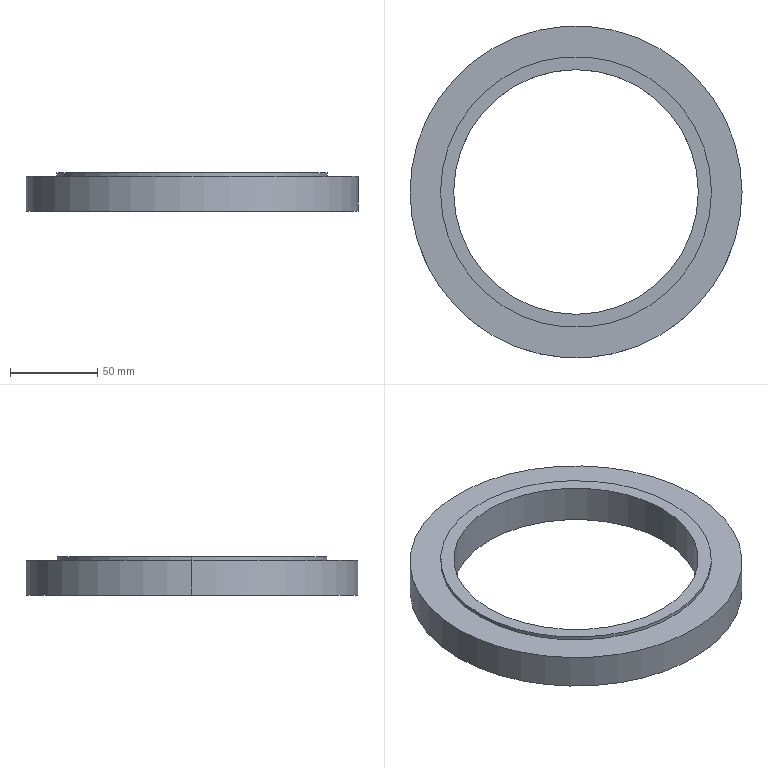Part | SolidWorks | features ICE 2, 3DProfileFeature 1, CirPattern 1, FlatPattern 1, HoleWzd 1, SMBaseFlange 1, SheetMetal 1 | 1 solid | 39 faces | box 190 x 190 x 22 mm | volume 258295 mm3 | cylinder 22 | cone 12 | plane 5 | commonest cylinder face diameters 6.8 x12 140 x2 148 x2 155 x2 156 x2 190 x2
STEP:
#1=CARTESIAN_POINT('',(-74.,0.,-17.8));
#2=VERTEX_POINT('',#1);
#3=CARTESIAN_POINT('',(74.,0.,-17.8));
#4=VERTEX_POINT('',#3);
#5=CARTESIAN_POINT('',(0.,0.,-17.8));
#6=DIRECTION('',(0.,0.,-1.));
#7=DIRECTION('',(-1.,0.,0.));
#8=AXIS2_PLACEMENT_3D('',#5,#6,#7);
#9=CIRCLE('',#8,74.);
#10=EDGE_CURVE('',#2,#4,#9,.T.);
#11=ORIENTED_EDGE('',*,*,#10,.T.);
#12=CARTESIAN_POINT('',(74.,0.,-20.));
#13=VERTEX_POINT('',#12);
#14=CARTESIAN_POINT('',(74.,0.,-17.8));
#15=DIRECTION('',(0.,0.,-1.));
#16=VECTOR('',#15,1000.);
#17=LINE('',#14,#16);
#18=EDGE_CURVE('',#4,#13,#17,.T.);
#19=ORIENTED_EDGE('',*,*,#18,.T.);
#20=CARTESIAN_POINT('',(-74.,0.,-20.));
#21=VERTEX_POINT('',#20);
#22=CARTESIAN_POINT('',(0.,0.,-20.));
#23=DIRECTION('',(0.,0.,-1.));
#24=DIRECTION('',(-1.,0.,0.));
#25=AXIS2_PLACEMENT_3D('',#22,#23,#24);
#26=CIRCLE('',#25,74.);
#27=EDGE_CURVE('',#21,#13,#26,.T.);
#28=ORIENTED_EDGE('',*,*,#27,.F.);
#29=CARTESIAN_POINT('',(-74.,0.,-17.8));
#30=DIRECTION('',(0.,0.,-1.));
#31=VECTOR('',#30,1000.);
#32=LINE('',#29,#31);
#33=EDGE_CURVE('',#2,#21,#32,.T.);
#34=ORIENTED_EDGE('',*,*,#33,.F.);
#35=EDGE_LOOP('',(#11,#19,#28,#34));
#36=FACE_OUTER_BOUND('',#35,.T.);
#37=CARTESIAN_POINT('',(0.,0.,-17.8));
#38=DIRECTION('',(0.,0.,-1.));
#39=DIRECTION('',(-1.,0.,0.));
#40=AXIS2_PLACEMENT_3D('',#37,#38,#39);
#41=CYLINDRICAL_SURFACE('',#40,74.);
#42=ADVANCED_FACE('',(#36),#41,.T.);
#43=CARTESIAN_POINT('',(78.,0.,-17.8));
#44=VERTEX_POINT('',#43);
#45=CARTESIAN_POINT('',(-78.,0.,-17.8));
#46=VERTEX_POINT('',#45);
#47=CARTESIAN_POINT('',(0.,0.,-17.8));
#48=DIRECTION('',(0.,0.,-1.));
#49=DIRECTION('',(-1.,0.,0.));
#50=AXIS2_PLACEMENT_3D('',#47,#48,#49);
#51=CIRCLE('',#50,78.);
#52=EDGE_CURVE('',#44,#46,#51,.T.);
#53=ORIENTED_EDGE('',*,*,#52,.F.);
#54=CARTESIAN_POINT('',(78.,0.,-20.));
#55=VERTEX_POINT('',#54);
#56=CARTESIAN_POINT('',(78.,0.,-17.8));
#57=DIRECTION('',(0.,0.,-1.));
#58=VECTOR('',#57,1000.);
#59=LINE('',#56,#58);
#60=EDGE_CURVE('',#44,#55,#59,.T.);
#61=ORIENTED_EDGE('',*,*,#60,.T.);
#62=CARTESIAN_POINT('',(-78.,0.,-20.));
#63=VERTEX_POINT('',#62);
#64=CARTESIAN_POINT('',(0.,0.,-20.));
#65=DIRECTION('',(0.,0.,-1.));
#66=DIRECTION('',(-1.,0.,0.));
#67=AXIS2_PLACEMENT_3D('',#64,#65,#66);
#68=CIRCLE('',#67,78.);
#69=EDGE_CURVE('',#55,#63,#68,.T.);
#70=ORIENTED_EDGE('',*,*,#69,.T.);
#71=CARTESIAN_POINT('',(-78.,0.,-17.8));
#72=DIRECTION('',(0.,0.,-1.));
#73=VECTOR('',#72,1000.);
#74=LINE('',#71,#73);
#75=EDGE_CURVE('',#46,#63,#74,.T.);
#76=ORIENTED_EDGE('',*,*,#75,.F.);
#77=EDGE_LOOP('',(#53,#61,#70,#76));
#78=FACE_OUTER_BOUND('',#77,.T.);
#79=CARTESIAN_POINT('',(0.,0.,-17.8));
#80=DIRECTION('',(0.,0.,-1.));
#81=DIRECTION('',(-1.,0.,0.));
#82=AXIS2_PLACEMENT_3D('',#79,#80,#81);
#83=CYLINDRICAL_SURFACE('',#82,78.);
#84=ADVANCED_FACE('',(#78),#83,.F.);
#85=CARTESIAN_POINT('',(46.4,-74.478,-4.));
#86=VERTEX_POINT('',#85);
#87=CARTESIAN_POINT('',(39.6,-74.478,-4.));
#88=VERTEX_POINT('',#87);
#89=CARTESIAN_POINT('',(43.,-74.478,-4.));
#90=DIRECTION('',(0.,0.,-1.));
#91=DIRECTION('',(-1.,0.,0.));
#92=AXIS2_PLACEMENT_3D('',#89,#90,#91);
#93=CIRCLE('',#92,3.4);
#94=EDGE_CURVE('',#86,#88,#93,.T.);
#95=ORIENTED_EDGE('',*,*,#94,.F.);
#96=CARTESIAN_POINT('',(46.4,-74.478,-20.));
#97=VERTEX_POINT('',#96);
#98=CARTESIAN_POINT('',(46.4,-74.478,-20.));
#99=DIRECTION('',(0.,0.,-1.));
#100=VECTOR('',#99,1000.);
#101=LINE('',#98,#100);
#102=EDGE_CURVE('',#86,#97,#101,.T.);
#103=ORIENTED_EDGE('',*,*,#102,.T.);
#104=CARTESIAN_POINT('',(39.6,-74.478,-20.));
#105=VERTEX_POINT('',#104);
#106=CARTESIAN_POINT('',(43.,-74.478,-20.));
#107=DIRECTION('',(0.,0.,-1.));
#108=DIRECTION('',(-1.,0.,0.));
#109=AXIS2_PLACEMENT_3D('',#106,#107,#108);
#110=CIRCLE('',#109,3.4);
#111=EDGE_CURVE('',#97,#105,#110,.T.);
#112=ORIENTED_EDGE('',*,*,#111,.T.);
#113=CARTESIAN_POINT('',(39.6,-74.478,-20.));
#114=DIRECTION('',(0.,0.,-1.));
#115=VECTOR('',#114,1000.);
#116=LINE('',#113,#115);
#117=EDGE_CURVE('',#88,#105,#116,.T.);
#118=ORIENTED_EDGE('',*,*,#117,.F.);
#119=EDGE_LOOP('',(#95,#103,#112,#118));
#120=FACE_OUTER_BOUND('',#119,.T.);
#121=CARTESIAN_POINT('',(43.,-74.478,-20.));
#122=DIRECTION('',(0.,0.,-1.));
#123=DIRECTION('',(-1.,0.,0.));
#124=AXIS2_PLACEMENT_3D('',#121,#122,#123);
#125=CYLINDRICAL_SURFACE('',#124,3.4);
#126=ADVANCED_FACE('',(#120),#125,.F.);
#127=CARTESIAN_POINT('',(43.,-74.478,-1.957));
#128=VERTEX_POINT('',#127);
#129=CARTESIAN_POINT('',(39.6,-74.478,-4.));
#130=DIRECTION('',(-0.8572,0.,-0.515));
#131=VECTOR('',#130,1000.);
#132=LINE('',#129,#131);
#133=EDGE_CURVE('',#128,#88,#132,.T.);
#134=ORIENTED_EDGE('',*,*,#133,.F.);
#135=CARTESIAN_POINT('',(46.4,-74.478,-4.));
#136=DIRECTION('',(0.8572,0.,-0.515));
#137=VECTOR('',#136,1000.);
#138=LINE('',#135,#137);
#139=EDGE_CURVE('',#128,#86,#138,.T.);
#140=ORIENTED_EDGE('',*,*,#139,.T.);
#141=ORIENTED_EDGE('',*,*,#94,.T.);
#142=EDGE_LOOP('',(#134,#140,#141));
#143=FACE_OUTER_BOUND('',#142,.T.);
#144=CARTESIAN_POINT('',(43.,-74.478,-4.));
#145=DIRECTION('',(0.,0.,-1.));
#146=DIRECTION('',(-1.,0.,0.));
#147=AXIS2_PLACEMENT_3D('',#144,#145,#146);
#148=CONICAL_SURFACE('',#147,3.4,1.03);
#149=ADVANCED_FACE('',(#143),#148,.F.);
#150=CARTESIAN_POINT('',(-39.6,-74.478,-4.));
#151=VERTEX_POINT('',#150);
#152=CARTESIAN_POINT('',(-46.4,-74.478,-4.));
#153=VERTEX_POINT('',#152);
#154=CARTESIAN_POINT('',(-43.,-74.478,-4.));
#155=DIRECTION('',(0.,0.,-1.));
#156=DIRECTION('',(-1.,0.,0.));
#157=AXIS2_PLACEMENT_3D('',#154,#155,#156);
#158=CIRCLE('',#157,3.4);
#159=EDGE_CURVE('',#151,#153,#158,.T.);
#160=ORIENTED_EDGE('',*,*,#159,.F.);
#161=CARTESIAN_POINT('',(-39.6,-74.478,-20.));
#162=VERTEX_POINT('',#161);
#163=CARTESIAN_POINT('',(-39.6,-74.478,-20.));
#164=DIRECTION('',(0.,0.,-1.));
#165=VECTOR('',#164,1000.);
#166=LINE('',#163,#165);
#167=EDGE_CURVE('',#151,#162,#166,.T.);
#168=ORIENTED_EDGE('',*,*,#167,.T.);
#169=CARTESIAN_POINT('',(-46.4,-74.478,-20.));
#170=VERTEX_POINT('',#169);
#171=CARTESIAN_POINT('',(-43.,-74.478,-20.));
#172=DIRECTION('',(0.,0.,-1.));
#173=DIRECTION('',(-1.,0.,0.));
#174=AXIS2_PLACEMENT_3D('',#171,#172,#173);
#175=CIRCLE('',#174,3.4);
#176=EDGE_CURVE('',#162,#170,#175,.T.);
#177=ORIENTED_EDGE('',*,*,#176,.T.);
#178=CARTESIAN_POINT('',(-46.4,-74.478,-20.));
#179=DIRECTION('',(0.,0.,-1.));
#180=VECTOR('',#179,1000.);
#181=LINE('',#178,#180);
#182=EDGE_CURVE('',#153,#170,#181,.T.);
#183=ORIENTED_EDGE('',*,*,#182,.F.);
#184=EDGE_LOOP('',(#160,#168,#177,#183));
#185=FACE_OUTER_BOUND('',#184,.T.);
#186=CARTESIAN_POINT('',(-43.,-74.478,-20.));
#187=DIRECTION('',(0.,0.,-1.));
#188=DIRECTION('',(-1.,0.,0.));
#189=AXIS2_PLACEMENT_3D('',#186,#187,#188);
#190=CYLINDRICAL_SURFACE('',#189,3.4);
#191=ADVANCED_FACE('',(#185),#190,.F.);
#192=CARTESIAN_POINT('',(-43.,-74.478,-1.957));
#193=VERTEX_POINT('',#192);
#194=CARTESIAN_POINT('',(-46.4,-74.478,-4.));
#195=DIRECTION('',(-0.8572,0.,-0.515));
#196=VECTOR('',#195,1000.);
#197=LINE('',#194,#196);
#198=EDGE_CURVE('',#193,#153,#197,.T.);
#199=ORIENTED_EDGE('',*,*,#198,.F.);
#200=CARTESIAN_POINT('',(-39.6,-74.478,-4.));
#201=DIRECTION('',(0.8572,0.,-0.515));
#202=VECTOR('',#201,1000.);
#203=LINE('',#200,#202);
#204=EDGE_CURVE('',#193,#151,#203,.T.);
#205=ORIENTED_EDGE('',*,*,#204,.T.);
#206=ORIENTED_EDGE('',*,*,#159,.T.);
#207=EDGE_LOOP('',(#199,#205,#206));
#208=FACE_OUTER_BOUND('',#207,.T.);
#209=CARTESIAN_POINT('',(-43.,-74.478,-4.));
#210=DIRECTION('',(0.,0.,-1.));
#211=DIRECTION('',(-1.,0.,0.));
#212=AXIS2_PLACEMENT_3D('',#209,#210,#211);
#213=CONICAL_SURFACE('',#212,3.4,1.03);
#214=ADVANCED_FACE('',(#208),#213,.F.);
#215=CARTESIAN_POINT('',(-82.6,0.,-4.));
#216=VERTEX_POINT('',#215);
#217=CARTESIAN_POINT('',(-89.4,0.,-4.));
#218=VERTEX_POINT('',#217);
#219=CARTESIAN_POINT('',(-86.,0.,-4.));
#220=DIRECTION('',(0.,0.,-1.));
#221=DIRECTION('',(-1.,0.,0.));
#222=AXIS2_PLACEMENT_3D('',#219,#220,#221);
#223=CIRCLE('',#222,3.4);
#224=EDGE_CURVE('',#216,#218,#223,.T.);
#225=ORIENTED_EDGE('',*,*,#224,.F.);
#226=CARTESIAN_POINT('',(-82.6,0.,-20.));
#227=VERTEX_POINT('',#226);
#228=CARTESIAN_POINT('',(-82.6,0.,-20.));
#229=DIRECTION('',(0.,0.,-1.));
#230=VECTOR('',#229,1000.);
#231=LINE('',#228,#230);
#232=EDGE_CURVE('',#216,#227,#231,.T.);
#233=ORIENTED_EDGE('',*,*,#232,.T.);
#234=CARTESIAN_POINT('',(-89.4,0.,-20.));
#235=VERTEX_POINT('',#234);
#236=CARTESIAN_POINT('',(-86.,0.,-20.));
#237=DIRECTION('',(0.,0.,-1.));
#238=DIRECTION('',(-1.,0.,0.));
#239=AXIS2_PLACEMENT_3D('',#236,#237,#238);
#240=CIRCLE('',#239,3.4);
#241=EDGE_CURVE('',#227,#235,#240,.T.);
#242=ORIENTED_EDGE('',*,*,#241,.T.);
#243=CARTESIAN_POINT('',(-89.4,0.,-20.));
#244=DIRECTION('',(0.,0.,-1.));
#245=VECTOR('',#244,1000.);
#246=LINE('',#243,#245);
#247=EDGE_CURVE('',#218,#235,#246,.T.);
#248=ORIENTED_EDGE('',*,*,#247,.F.);
#249=EDGE_LOOP('',(#225,#233,#242,#248));
#250=FACE_OUTER_BOUND('',#249,.T.);
#251=CARTESIAN_POINT('',(-86.,0.,-20.));
#252=DIRECTION('',(0.,0.,-1.));
#253=DIRECTION('',(-1.,0.,0.));
#254=AXIS2_PLACEMENT_3D('',#251,#252,#253);
#255=CYLINDRICAL_SURFACE('',#254,3.4);
#256=ADVANCED_FACE('',(#250),#255,.F.);
#257=CARTESIAN_POINT('',(-86.,0.,-1.957));
#258=VERTEX_POINT('',#257);
#259=CARTESIAN_POINT('',(-89.4,0.,-4.));
#260=DIRECTION('',(-0.8572,0.,-0.515));
#261=VECTOR('',#260,1000.);
#262=LINE('',#259,#261);
#263=EDGE_CURVE('',#258,#218,#262,.T.);
#264=ORIENTED_EDGE('',*,*,#263,.F.);
#265=CARTESIAN_POINT('',(-82.6,0.,-4.));
#266=DIRECTION('',(0.8572,0.,-0.515));
#267=VECTOR('',#266,1000.);
#268=LINE('',#265,#267);
#269=EDGE_CURVE('',#258,#216,#268,.T.);
#270=ORIENTED_EDGE('',*,*,#269,.T.);
#271=ORIENTED_EDGE('',*,*,#224,.T.);
#272=EDGE_LOOP('',(#264,#270,#271));
#273=FACE_OUTER_BOUND('',#272,.T.);
#274=CARTESIAN_POINT('',(-86.,0.,-4.));
#275=DIRECTION('',(0.,0.,-1.));
#276=DIRECTION('',(-1.,0.,0.));
#277=AXIS2_PLACEMENT_3D('',#274,#275,#276);
#278=CONICAL_SURFACE('',#277,3.4,1.03);
#279=ADVANCED_FACE('',(#273),#278,.F.);
#280=CARTESIAN_POINT('',(-39.6,74.478,-4.));
#281=VERTEX_POINT('',#280);
#282=CARTESIAN_POINT('',(-46.4,74.478,-4.));
#283=VERTEX_POINT('',#282);
#284=CARTESIAN_POINT('',(-43.,74.478,-4.));
#285=DIRECTION('',(0.,0.,-1.));
#286=DIRECTION('',(-1.,0.,0.));
#287=AXIS2_PLACEMENT_3D('',#284,#285,#286);
#288=CIRCLE('',#287,3.4);
#289=EDGE_CURVE('',#281,#283,#288,.T.);
#290=ORIENTED_EDGE('',*,*,#289,.F.);
#291=CARTESIAN_POINT('',(-39.6,74.478,-20.));
#292=VERTEX_POINT('',#291);
#293=CARTESIAN_POINT('',(-39.6,74.478,-20.));
#294=DIRECTION('',(0.,0.,-1.));
#295=VECTOR('',#294,1000.);
#296=LINE('',#293,#295);
#297=EDGE_CURVE('',#281,#292,#296,.T.);
#298=ORIENTED_EDGE('',*,*,#297,.T.);
#299=CARTESIAN_POINT('',(-46.4,74.478,-20.));
#300=VERTEX_POINT('',#299);
#301=CARTESIAN_POINT('',(-43.,74.478,-20.));
#302=DIRECTION('',(0.,0.,-1.));
#303=DIRECTION('',(-1.,0.,0.));
#304=AXIS2_PLACEMENT_3D('',#301,#302,#303);
#305=CIRCLE('',#304,3.4);
#306=EDGE_CURVE('',#292,#300,#305,.T.);
#307=ORIENTED_EDGE('',*,*,#306,.T.);
#308=CARTESIAN_POINT('',(-46.4,74.478,-20.));
#309=DIRECTION('',(0.,0.,-1.));
#310=VECTOR('',#309,1000.);
#311=LINE('',#308,#310);
#312=EDGE_CURVE('',#283,#300,#311,.T.);
#313=ORIENTED_EDGE('',*,*,#312,.F.);
#314=EDGE_LOOP('',(#290,#298,#307,#313));
#315=FACE_OUTER_BOUND('',#314,.T.);
#316=CARTESIAN_POINT('',(-43.,74.478,-20.));
#317=DIRECTION('',(0.,0.,-1.));
#318=DIRECTION('',(-1.,0.,0.));
#319=AXIS2_PLACEMENT_3D('',#316,#317,#318);
#320=CYLINDRICAL_SURFACE('',#319,3.4);
#321=ADVANCED_FACE('',(#315),#320,.F.);
#322=CARTESIAN_POINT('',(-43.,74.478,-1.957));
#323=VERTEX_POINT('',#322);
#324=CARTESIAN_POINT('',(-46.4,74.478,-4.));
#325=DIRECTION('',(-0.8572,0.,-0.515));
#326=VECTOR('',#325,1000.);
#327=LINE('',#324,#326);
#328=EDGE_CURVE('',#323,#283,#327,.T.);
#329=ORIENTED_EDGE('',*,*,#328,.F.);
#330=CARTESIAN_POINT('',(-39.6,74.478,-4.));
#331=DIRECTION('',(0.8572,0.,-0.515));
#332=VECTOR('',#331,1000.);
#333=LINE('',#330,#332);
#334=EDGE_CURVE('',#323,#281,#333,.T.);
#335=ORIENTED_EDGE('',*,*,#334,.T.);
#336=ORIENTED_EDGE('',*,*,#289,.T.);
#337=EDGE_LOOP('',(#329,#335,#336));
#338=FACE_OUTER_BOUND('',#337,.T.);
#339=CARTESIAN_POINT('',(-43.,74.478,-4.));
#340=DIRECTION('',(0.,0.,-1.));
#341=DIRECTION('',(-1.,0.,0.));
#342=AXIS2_PLACEMENT_3D('',#339,#340,#341);
#343=CONICAL_SURFACE('',#342,3.4,1.03);
#344=ADVANCED_FACE('',(#338),#343,.F.);
#345=CARTESIAN_POINT('',(46.4,74.478,-4.));
#346=VERTEX_POINT('',#345);
#347=CARTESIAN_POINT('',(39.6,74.478,-4.));
#348=VERTEX_POINT('',#347);
#349=CARTESIAN_POINT('',(43.,74.478,-4.));
#350=DIRECTION('',(0.,0.,-1.));
#351=DIRECTION('',(-1.,0.,0.));
#352=AXIS2_PLACEMENT_3D('',#349,#350,#351);
#353=CIRCLE('',#352,3.4);
#354=EDGE_CURVE('',#346,#348,#353,.T.);
#355=ORIENTED_EDGE('',*,*,#354,.F.);
#356=CARTESIAN_POINT('',(46.4,74.478,-20.));
#357=VERTEX_POINT('',#356);
#358=CARTESIAN_POINT('',(46.4,74.478,-20.));
#359=DIRECTION('',(0.,0.,-1.));
#360=VECTOR('',#359,1000.);
#361=LINE('',#358,#360);
#362=EDGE_CURVE('',#346,#357,#361,.T.);
#363=ORIENTED_EDGE('',*,*,#362,.T.);
#364=CARTESIAN_POINT('',(39.6,74.478,-20.));
#365=VERTEX_POINT('',#364);
#366=CARTESIAN_POINT('',(43.,74.478,-20.));
#367=DIRECTION('',(0.,0.,-1.));
#368=DIRECTION('',(-1.,0.,0.));
#369=AXIS2_PLACEMENT_3D('',#366,#367,#368);
#370=CIRCLE('',#369,3.4);
#371=EDGE_CURVE('',#357,#365,#370,.T.);
#372=ORIENTED_EDGE('',*,*,#371,.T.);
#373=CARTESIAN_POINT('',(39.6,74.478,-20.));
#374=DIRECTION('',(0.,0.,-1.));
#375=VECTOR('',#374,1000.);
#376=LINE('',#373,#375);
#377=EDGE_CURVE('',#348,#365,#376,.T.);
#378=ORIENTED_EDGE('',*,*,#377,.F.);
#379=EDGE_LOOP('',(#355,#363,#372,#378));
#380=FACE_OUTER_BOUND('',#379,.T.);
#381=CARTESIAN_POINT('',(43.,74.478,-20.));
#382=DIRECTION('',(0.,0.,-1.));
#383=DIRECTION('',(-1.,0.,0.));
#384=AXIS2_PLACEMENT_3D('',#381,#382,#383);
#385=CYLINDRICAL_SURFACE('',#384,3.4);
#386=ADVANCED_FACE('',(#380),#385,.F.);
#387=CARTESIAN_POINT('',(43.,74.478,-1.957));
#388=VERTEX_POINT('',#387);
#389=CARTESIAN_POINT('',(39.6,74.478,-4.));
#390=DIRECTION('',(-0.8572,0.,-0.515));
#391=VECTOR('',#390,1000.);
#392=LINE('',#389,#391);
#393=EDGE_CURVE('',#388,#348,#392,.T.);
#394=ORIENTED_EDGE('',*,*,#393,.F.);
#395=CARTESIAN_POINT('',(46.4,74.478,-4.));
#396=DIRECTION('',(0.8572,0.,-0.515));
#397=VECTOR('',#396,1000.);
#398=LINE('',#395,#397);
#399=EDGE_CURVE('',#388,#346,#398,.T.);
#400=ORIENTED_EDGE('',*,*,#399,.T.);
#401=ORIENTED_EDGE('',*,*,#354,.T.);
#402=EDGE_LOOP('',(#394,#400,#401));
#403=FACE_OUTER_BOUND('',#402,.T.);
#404=CARTESIAN_POINT('',(43.,74.478,-4.));
#405=DIRECTION('',(0.,0.,-1.));
#406=DIRECTION('',(-1.,0.,0.));
#407=AXIS2_PLACEMENT_3D('',#404,#405,#406);
#408=CONICAL_SURFACE('',#407,3.4,1.03);
#409=ADVANCED_FACE('',(#403),#408,.F.);
#410=CARTESIAN_POINT('',(89.4,0.,-4.));
#411=VERTEX_POINT('',#410);
#412=CARTESIAN_POINT('',(82.6,0.,-4.));
#413=VERTEX_POINT('',#412);
#414=CARTESIAN_POINT('',(86.,0.,-4.));
#415=DIRECTION('',(0.,0.,-1.));
#416=DIRECTION('',(-1.,0.,0.));
#417=AXIS2_PLACEMENT_3D('',#414,#415,#416);
#418=CIRCLE('',#417,3.4);
#419=EDGE_CURVE('',#411,#413,#418,.T.);
#420=ORIENTED_EDGE('',*,*,#419,.F.);
#421=CARTESIAN_POINT('',(89.4,0.,-20.));
#422=VERTEX_POINT('',#421);
#423=CARTESIAN_POINT('',(89.4,0.,-20.));
#424=DIRECTION('',(0.,0.,-1.));
#425=VECTOR('',#424,1000.);
#426=LINE('',#423,#425);
#427=EDGE_CURVE('',#411,#422,#426,.T.);
#428=ORIENTED_EDGE('',*,*,#427,.T.);
#429=CARTESIAN_POINT('',(82.6,0.,-20.));
#430=VERTEX_POINT('',#429);
#431=CARTESIAN_POINT('',(86.,0.,-20.));
#432=DIRECTION('',(0.,0.,-1.));
#433=DIRECTION('',(-1.,0.,0.));
#434=AXIS2_PLACEMENT_3D('',#431,#432,#433);
#435=CIRCLE('',#434,3.4);
#436=EDGE_CURVE('',#422,#430,#435,.T.);
#437=ORIENTED_EDGE('',*,*,#436,.T.);
#438=CARTESIAN_POINT('',(82.6,0.,-20.));
#439=DIRECTION('',(0.,0.,-1.));
#440=VECTOR('',#439,1000.);
#441=LINE('',#438,#440);
#442=EDGE_CURVE('',#413,#430,#441,.T.);
#443=ORIENTED_EDGE('',*,*,#442,.F.);
#444=EDGE_LOOP('',(#420,#428,#437,#443));
#445=FACE_OUTER_BOUND('',#444,.T.);
#446=CARTESIAN_POINT('',(86.,0.,-20.));
#447=DIRECTION('',(0.,0.,-1.));
#448=DIRECTION('',(-1.,0.,0.));
#449=AXIS2_PLACEMENT_3D('',#446,#447,#448);
#450=CYLINDRICAL_SURFACE('',#449,3.4);
#451=ADVANCED_FACE('',(#445),#450,.F.);
#452=CARTESIAN_POINT('',(86.,0.,-1.957));
#453=VERTEX_POINT('',#452);
#454=CARTESIAN_POINT('',(82.6,0.,-4.));
#455=DIRECTION('',(-0.8572,0.,-0.515));
#456=VECTOR('',#455,1000.);
#457=LINE('',#454,#456);
#458=EDGE_CURVE('',#453,#413,#457,.T.);
#459=ORIENTED_EDGE('',*,*,#458,.F.);
#460=CARTESIAN_POINT('',(89.4,0.,-4.));
#461=DIRECTION('',(0.8572,0.,-0.515));
#462=VECTOR('',#461,1000.);
#463=LINE('',#460,#462);
#464=EDGE_CURVE('',#453,#411,#463,.T.);
#465=ORIENTED_EDGE('',*,*,#464,.T.);
#466=ORIENTED_EDGE('',*,*,#419,.T.);
#467=EDGE_LOOP('',(#459,#465,#466));
#468=FACE_OUTER_BOUND('',#467,.T.);
#469=CARTESIAN_POINT('',(86.,0.,-4.));
#470=DIRECTION('',(0.,0.,-1.));
#471=DIRECTION('',(-1.,0.,0.));
#472=AXIS2_PLACEMENT_3D('',#469,#470,#471);
#473=CONICAL_SURFACE('',#472,3.4,1.03);
#474=ADVANCED_FACE('',(#468),#473,.F.);
#475=CARTESIAN_POINT('',(77.5,0.,2.));
#476=VERTEX_POINT('',#475);
#477=CARTESIAN_POINT('',(-77.5,0.,2.));
#478=VERTEX_POINT('',#477);
#479=CARTESIAN_POINT('',(0.,0.,2.));
#480=DIRECTION('',(0.,0.,1.));
#481=DIRECTION('',(1.,0.,0.));
#482=AXIS2_PLACEMENT_3D('',#479,#480,#481);
#483=CIRCLE('',#482,77.5);
#484=EDGE_CURVE('',#476,#478,#483,.T.);
#485=ORIENTED_EDGE('',*,*,#484,.F.);
#486=CARTESIAN_POINT('',(77.5,0.,0.));
#487=VERTEX_POINT('',#486);
#488=CARTESIAN_POINT('',(77.5,0.,2.));
#489=DIRECTION('',(0.,0.,-1.));
#490=VECTOR('',#489,1000.);
#491=LINE('',#488,#490);
#492=EDGE_CURVE('',#476,#487,#491,.T.);
#493=ORIENTED_EDGE('',*,*,#492,.T.);
#494=CARTESIAN_POINT('',(-77.5,0.,0.));
#495=VERTEX_POINT('',#494);
#496=CARTESIAN_POINT('',(0.,0.,0.));
#497=DIRECTION('',(0.,0.,1.));
#498=DIRECTION('',(1.,0.,0.));
#499=AXIS2_PLACEMENT_3D('',#496,#497,#498);
#500=CIRCLE('',#499,77.5);
#501=EDGE_CURVE('',#487,#495,#500,.T.);
#502=ORIENTED_EDGE('',*,*,#501,.T.);
#503=CARTESIAN_POINT('',(-77.5,0.,2.));
#504=DIRECTION('',(0.,0.,-1.));
#505=VECTOR('',#504,1000.);
#506=LINE('',#503,#505);
#507=EDGE_CURVE('',#478,#495,#506,.T.);
#508=ORIENTED_EDGE('',*,*,#507,.F.);
#509=EDGE_LOOP('',(#485,#493,#502,#508));
#510=FACE_OUTER_BOUND('',#509,.T.);
#511=CARTESIAN_POINT('',(0.,0.,2.));
#512=DIRECTION('',(0.,0.,-1.));
#513=DIRECTION('',(-1.,0.,0.));
#514=AXIS2_PLACEMENT_3D('',#511,#512,#513);
#515=CYLINDRICAL_SURFACE('',#514,77.5);
#516=ADVANCED_FACE('',(#510),#515,.T.);
#517=CARTESIAN_POINT('',(-70.,0.,-20.));
#518=VERTEX_POINT('',#517);
#519=CARTESIAN_POINT('',(70.,0.,-20.));
#520=VERTEX_POINT('',#519);
#521=CARTESIAN_POINT('',(0.,0.,-20.));
#522=DIRECTION('',(0.,0.,1.));
#523=DIRECTION('',(1.,0.,0.));
#524=AXIS2_PLACEMENT_3D('',#521,#522,#523);
#525=CIRCLE('',#524,70.);
#526=EDGE_CURVE('',#518,#520,#525,.T.);
#527=ORIENTED_EDGE('',*,*,#526,.F.);
#528=CARTESIAN_POINT('',(-70.,0.,2.));
#529=VERTEX_POINT('',#528);
#530=CARTESIAN_POINT('',(-70.,0.,-20.));
#531=DIRECTION('',(0.,0.,1.));
#532=VECTOR('',#531,1000.);
#533=LINE('',#530,#532);
#534=EDGE_CURVE('',#518,#529,#533,.T.);
#535=ORIENTED_EDGE('',*,*,#534,.T.);
#536=CARTESIAN_POINT('',(70.,0.,2.));
#537=VERTEX_POINT('',#536);
#538=CARTESIAN_POINT('',(0.,0.,2.));
#539=DIRECTION('',(0.,0.,1.));
#540=DIRECTION('',(1.,0.,0.));
#541=AXIS2_PLACEMENT_3D('',#538,#539,#540);
#542=CIRCLE('',#541,70.);
#543=EDGE_CURVE('',#529,#537,#542,.T.);
#544=ORIENTED_EDGE('',*,*,#543,.T.);
#545=CARTESIAN_POINT('',(70.,0.,-20.));
#546=DIRECTION('',(0.,0.,1.));
#547=VECTOR('',#546,1000.);
#548=LINE('',#545,#547);
#549=EDGE_CURVE('',#520,#537,#548,.T.);
#550=ORIENTED_EDGE('',*,*,#549,.F.);
#551=EDGE_LOOP('',(#527,#535,#544,#550));
#552=FACE_OUTER_BOUND('',#551,.T.);
#553=CARTESIAN_POINT('',(0.,0.,-20.));
#554=DIRECTION('',(0.,0.,1.));
#555=DIRECTION('',(1.,0.,0.));
#556=AXIS2_PLACEMENT_3D('',#553,#554,#555);
#557=CYLINDRICAL_SURFACE('',#556,70.);
#558=ADVANCED_FACE('',(#552),#557,.F.);
#559=CARTESIAN_POINT('',(95.,0.,-20.));
#560=VERTEX_POINT('',#559);
#561=CARTESIAN_POINT('',(-95.,0.,-20.));
#562=VERTEX_POINT('',#561);
#563=CARTESIAN_POINT('',(0.,0.,-20.));
#564=DIRECTION('',(0.,0.,1.));
#565=DIRECTION('',(1.,0.,0.));
#566=AXIS2_PLACEMENT_3D('',#563,#564,#565);
#567=CIRCLE('',#566,95.);
#568=EDGE_CURVE('',#560,#562,#567,.T.);
#569=ORIENTED_EDGE('',*,*,#568,.T.);
#570=CARTESIAN_POINT('',(-95.,0.,0.));
#571=VERTEX_POINT('',#570);
#572=CARTESIAN_POINT('',(-95.,0.,-20.));
#573=DIRECTION('',(0.,0.,1.));
#574=VECTOR('',#573,1000.);
#575=LINE('',#572,#574);
#576=EDGE_CURVE('',#562,#571,#575,.T.);
#577=ORIENTED_EDGE('',*,*,#576,.T.);
#578=CARTESIAN_POINT('',(95.,0.,0.));
#579=VERTEX_POINT('',#578);
#580=CARTESIAN_POINT('',(0.,0.,0.));
#581=DIRECTION('',(0.,0.,1.));
#582=DIRECTION('',(1.,0.,0.));
#583=AXIS2_PLACEMENT_3D('',#580,#581,#582);
#584=CIRCLE('',#583,95.);
#585=EDGE_CURVE('',#579,#571,#584,.T.);
#586=ORIENTED_EDGE('',*,*,#585,.F.);
#587=CARTESIAN_POINT('',(95.,0.,-20.));
#588=DIRECTION('',(0.,0.,1.));
#589=VECTOR('',#588,1000.);
#590=LINE('',#587,#589);
#591=EDGE_CURVE('',#560,#579,#590,.T.);
#592=ORIENTED_EDGE('',*,*,#591,.F.);
#593=EDGE_LOOP('',(#569,#577,#586,#592));
#594=FACE_OUTER_BOUND('',#593,.T.);
#595=CARTESIAN_POINT('',(0.,0.,-20.));
#596=DIRECTION('',(0.,0.,1.));
#597=DIRECTION('',(1.,0.,0.));
#598=AXIS2_PLACEMENT_3D('',#595,#596,#597);
#599=CYLINDRICAL_SURFACE('',#598,95.);
#600=ADVANCED_FACE('',(#594),#599,.T.);
#601=CARTESIAN_POINT('',(0.,0.,-20.));
#602=DIRECTION('',(0.,0.,1.));
#603=DIRECTION('',(1.,0.,0.));
#604=AXIS2_PLACEMENT_3D('',#601,#602,#603);
#605=CIRCLE('',#604,70.);
#606=EDGE_CURVE('',#520,#518,#605,.T.);
#607=ORIENTED_EDGE('',*,*,#606,.T.);
#608=ORIENTED_EDGE('',*,*,#526,.T.);
#609=EDGE_LOOP('',(#607,#608));
#610=FACE_BOUND('',#609,.T.);
#611=ORIENTED_EDGE('',*,*,#27,.T.);
#612=CARTESIAN_POINT('',(0.,0.,-20.));
#613=DIRECTION('',(0.,0.,-1.));
#614=DIRECTION('',(-1.,0.,0.));
#615=AXIS2_PLACEMENT_3D('',#612,#613,#614);
#616=CIRCLE('',#615,74.);
#617=EDGE_CURVE('',#13,#21,#616,.T.);
#618=ORIENTED_EDGE('',*,*,#617,.T.);
#619=EDGE_LOOP('',(#611,#618));
#620=FACE_OUTER_BOUND('',#619,.T.);
#621=CARTESIAN_POINT('',(0.,0.,-20.));
#622=DIRECTION('',(0.,0.,1.));
#623=DIRECTION('',(1.,0.,0.));
#624=AXIS2_PLACEMENT_3D('',#621,#622,#623);
#625=PLANE('',#624);
#626=ADVANCED_FACE('',(#610,#620),#625,.F.);
#627=ORIENTED_EDGE('',*,*,#585,.T.);
#628=CARTESIAN_POINT('',(0.,0.,0.));
#629=DIRECTION('',(0.,0.,1.));
#630=DIRECTION('',(1.,0.,0.));
#631=AXIS2_PLACEMENT_3D('',#628,#629,#630);
#632=CIRCLE('',#631,95.);
#633=EDGE_CURVE('',#571,#579,#632,.T.);
#634=ORIENTED_EDGE('',*,*,#633,.T.);
#635=EDGE_LOOP('',(#627,#634));
#636=FACE_OUTER_BOUND('',#635,.T.);
#637=CARTESIAN_POINT('',(0.,0.,0.));
#638=DIRECTION('',(0.,0.,1.));
#639=DIRECTION('',(1.,0.,0.));
#640=AXIS2_PLACEMENT_3D('',#637,#638,#639);
#641=CIRCLE('',#640,77.5);
#642=EDGE_CURVE('',#495,#487,#641,.T.);
#643=ORIENTED_EDGE('',*,*,#642,.F.);
#644=ORIENTED_EDGE('',*,*,#501,.F.);
#645=EDGE_LOOP('',(#643,#644));
#646=FACE_BOUND('',#645,.T.);
#647=CARTESIAN_POINT('',(0.,0.,0.));
#648=DIRECTION('',(0.,0.,1.));
#649=DIRECTION('',(1.,0.,0.));
#650=AXIS2_PLACEMENT_3D('',#647,#648,#649);
#651=PLANE('',#650);
#652=ADVANCED_FACE('',(#636,#646),#651,.T.);
#653=ORIENTED_EDGE('',*,*,#576,.F.);
#654=CARTESIAN_POINT('',(0.,0.,-20.));
#655=DIRECTION('',(0.,0.,1.));
#656=DIRECTION('',(1.,0.,0.));
#657=AXIS2_PLACEMENT_3D('',#654,#655,#656);
#658=CIRCLE('',#657,95.);
#659=EDGE_CURVE('',#562,#560,#658,.T.);
#660=ORIENTED_EDGE('',*,*,#659,.T.);
#661=ORIENTED_EDGE('',*,*,#591,.T.);
#662=ORIENTED_EDGE('',*,*,#633,.F.);
#663=EDGE_LOOP('',(#653,#660,#661,#662));
#664=FACE_OUTER_BOUND('',#663,.T.);
#665=CARTESIAN_POINT('',(0.,0.,-20.));
#666=DIRECTION('',(0.,0.,1.));
#667=DIRECTION('',(1.,0.,0.));
#668=AXIS2_PLACEMENT_3D('',#665,#666,#667);
#669=CYLINDRICAL_SURFACE('',#668,95.);
#670=ADVANCED_FACE('',(#664),#669,.T.);
#671=CARTESIAN_POINT('',(0.,0.,-20.));
#672=DIRECTION('',(0.,0.,-1.));
#673=DIRECTION('',(-1.,0.,0.));
#674=AXIS2_PLACEMENT_3D('',#671,#672,#673);
#675=CIRCLE('',#674,78.);
#676=EDGE_CURVE('',#63,#55,#675,.T.);
#677=ORIENTED_EDGE('',*,*,#676,.F.);
#678=ORIENTED_EDGE('',*,*,#69,.F.);
#679=EDGE_LOOP('',(#677,#678));
#680=FACE_BOUND('',#679,.T.);
#681=CARTESIAN_POINT('',(43.,-74.478,-20.));
#682=DIRECTION('',(0.,0.,-1.));
#683=DIRECTION('',(-1.,0.,0.));
#684=AXIS2_PLACEMENT_3D('',#681,#682,#683);
#685=CIRCLE('',#684,3.4);
#686=EDGE_CURVE('',#105,#97,#685,.T.);
#687=ORIENTED_EDGE('',*,*,#686,.F.);
#688=ORIENTED_EDGE('',*,*,#111,.F.);
#689=EDGE_LOOP('',(#687,#688));
#690=FACE_BOUND('',#689,.T.);
#691=CARTESIAN_POINT('',(-43.,-74.478,-20.));
#692=DIRECTION('',(0.,0.,-1.));
#693=DIRECTION('',(-1.,0.,0.));
#694=AXIS2_PLACEMENT_3D('',#691,#692,#693);
#695=CIRCLE('',#694,3.4);
#696=EDGE_CURVE('',#170,#162,#695,.T.);
#697=ORIENTED_EDGE('',*,*,#696,.F.);
#698=ORIENTED_EDGE('',*,*,#176,.F.);
#699=EDGE_LOOP('',(#697,#698));
#700=FACE_BOUND('',#699,.T.);
#701=CARTESIAN_POINT('',(-86.,0.,-20.));
#702=DIRECTION('',(0.,0.,-1.));
#703=DIRECTION('',(-1.,0.,0.));
#704=AXIS2_PLACEMENT_3D('',#701,#702,#703);
#705=CIRCLE('',#704,3.4);
#706=EDGE_CURVE('',#235,#227,#705,.T.);
#707=ORIENTED_EDGE('',*,*,#706,.F.);
#708=ORIENTED_EDGE('',*,*,#241,.F.);
#709=EDGE_LOOP('',(#707,#708));
#710=FACE_BOUND('',#709,.T.);
#711=CARTESIAN_POINT('',(-43.,74.478,-20.));
#712=DIRECTION('',(0.,0.,-1.));
#713=DIRECTION('',(-1.,0.,0.));
#714=AXIS2_PLACEMENT_3D('',#711,#712,#713);
#715=CIRCLE('',#714,3.4);
#716=EDGE_CURVE('',#300,#292,#715,.T.);
#717=ORIENTED_EDGE('',*,*,#716,.F.);
#718=ORIENTED_EDGE('',*,*,#306,.F.);
#719=EDGE_LOOP('',(#717,#718));
#720=FACE_BOUND('',#719,.T.);
#721=CARTESIAN_POINT('',(43.,74.478,-20.));
#722=DIRECTION('',(0.,0.,-1.));
#723=DIRECTION('',(-1.,0.,0.));
#724=AXIS2_PLACEMENT_3D('',#721,#722,#723);
#725=CIRCLE('',#724,3.4);
#726=EDGE_CURVE('',#365,#357,#725,.T.);
#727=ORIENTED_EDGE('',*,*,#726,.F.);
#728=ORIENTED_EDGE('',*,*,#371,.F.);
#729=EDGE_LOOP('',(#727,#728));
#730=FACE_BOUND('',#729,.T.);
#731=CARTESIAN_POINT('',(86.,0.,-20.));
#732=DIRECTION('',(0.,0.,-1.));
#733=DIRECTION('',(-1.,0.,0.));
#734=AXIS2_PLACEMENT_3D('',#731,#732,#733);
#735=CIRCLE('',#734,3.4);
#736=EDGE_CURVE('',#430,#422,#735,.T.);
#737=ORIENTED_EDGE('',*,*,#736,.F.);
#738=ORIENTED_EDGE('',*,*,#436,.F.);
#739=EDGE_LOOP('',(#737,#738));
#740=FACE_BOUND('',#739,.T.);
#741=ORIENTED_EDGE('',*,*,#568,.F.);
#742=ORIENTED_EDGE('',*,*,#659,.F.);
#743=EDGE_LOOP('',(#741,#742));
#744=FACE_OUTER_BOUND('',#743,.T.);
#745=CARTESIAN_POINT('',(0.,0.,-20.));
#746=DIRECTION('',(0.,0.,1.));
#747=DIRECTION('',(1.,0.,0.));
#748=AXIS2_PLACEMENT_3D('',#745,#746,#747);
#749=PLANE('',#748);
#750=ADVANCED_FACE('',(#680,#690,#700,#710,#720,#730,#740,#744),#749,.F.);
#751=ORIENTED_EDGE('',*,*,#534,.F.);
#752=ORIENTED_EDGE('',*,*,#606,.F.);
#753=ORIENTED_EDGE('',*,*,#549,.T.);
#754=CARTESIAN_POINT('',(0.,0.,2.));
#755=DIRECTION('',(0.,0.,1.));
#756=DIRECTION('',(1.,0.,0.));
#757=AXIS2_PLACEMENT_3D('',#754,#755,#756);
#758=CIRCLE('',#757,70.);
#759=EDGE_CURVE('',#537,#529,#758,.T.);
#760=ORIENTED_EDGE('',*,*,#759,.T.);
#761=EDGE_LOOP('',(#751,#752,#753,#760));
#762=FACE_OUTER_BOUND('',#761,.T.);
#763=CARTESIAN_POINT('',(0.,0.,-20.));
#764=DIRECTION('',(0.,0.,1.));
#765=DIRECTION('',(1.,0.,0.));
#766=AXIS2_PLACEMENT_3D('',#763,#764,#765);
#767=CYLINDRICAL_SURFACE('',#766,70.);
#768=ADVANCED_FACE('',(#762),#767,.F.);
#769=CARTESIAN_POINT('',(0.,0.,2.));
#770=DIRECTION('',(0.,0.,1.));
#771=DIRECTION('',(1.,0.,0.));
#772=AXIS2_PLACEMENT_3D('',#769,#770,#771);
#773=CIRCLE('',#772,77.5);
#774=EDGE_CURVE('',#478,#476,#773,.T.);
#775=ORIENTED_EDGE('',*,*,#774,.T.);
#776=ORIENTED_EDGE('',*,*,#484,.T.);
#777=EDGE_LOOP('',(#775,#776));
#778=FACE_OUTER_BOUND('',#777,.T.);
#779=ORIENTED_EDGE('',*,*,#759,.F.);
#780=ORIENTED_EDGE('',*,*,#543,.F.);
#781=EDGE_LOOP('',(#779,#780));
#782=FACE_BOUND('',#781,.T.);
#783=CARTESIAN_POINT('',(0.,0.,2.));
#784=DIRECTION('',(0.,0.,1.));
#785=DIRECTION('',(1.,0.,0.));
#786=AXIS2_PLACEMENT_3D('',#783,#784,#785);
#787=PLANE('',#786);
#788=ADVANCED_FACE('',(#778,#782),#787,.T.);
#789=ORIENTED_EDGE('',*,*,#492,.F.);
#790=ORIENTED_EDGE('',*,*,#774,.F.);
#791=ORIENTED_EDGE('',*,*,#507,.T.);
#792=ORIENTED_EDGE('',*,*,#642,.T.);
#793=EDGE_LOOP('',(#789,#790,#791,#792));
#794=FACE_OUTER_BOUND('',#793,.T.);
#795=CARTESIAN_POINT('',(0.,0.,2.));
#796=DIRECTION('',(0.,0.,-1.));
#797=DIRECTION('',(-1.,0.,0.));
#798=AXIS2_PLACEMENT_3D('',#795,#796,#797);
#799=CYLINDRICAL_SURFACE('',#798,77.5);
#800=ADVANCED_FACE('',(#794),#799,.T.);
#801=ORIENTED_EDGE('',*,*,#464,.F.);
#802=ORIENTED_EDGE('',*,*,#458,.T.);
#803=CARTESIAN_POINT('',(86.,0.,-4.));
#804=DIRECTION('',(0.,0.,-1.));
#805=DIRECTION('',(-1.,0.,0.));
#806=AXIS2_PLACEMENT_3D('',#803,#804,#805);
#807=CIRCLE('',#806,3.4);
#808=EDGE_CURVE('',#413,#411,#807,.T.);
#809=ORIENTED_EDGE('',*,*,#808,.T.);
#810=EDGE_LOOP('',(#801,#802,#809));
#811=FACE_OUTER_BOUND('',#810,.T.);
#812=CARTESIAN_POINT('',(86.,0.,-4.));
#813=DIRECTION('',(0.,0.,-1.));
#814=DIRECTION('',(-1.,0.,0.));
#815=AXIS2_PLACEMENT_3D('',#812,#813,#814);
#816=CONICAL_SURFACE('',#815,3.4,1.03);
#817=ADVANCED_FACE('',(#811),#816,.F.);
#818=ORIENTED_EDGE('',*,*,#427,.F.);
#819=ORIENTED_EDGE('',*,*,#808,.F.);
#820=ORIENTED_EDGE('',*,*,#442,.T.);
#821=ORIENTED_EDGE('',*,*,#736,.T.);
#822=EDGE_LOOP('',(#818,#819,#820,#821));
#823=FACE_OUTER_BOUND('',#822,.T.);
#824=CARTESIAN_POINT('',(86.,0.,-20.));
#825=DIRECTION('',(0.,0.,-1.));
#826=DIRECTION('',(-1.,0.,0.));
#827=AXIS2_PLACEMENT_3D('',#824,#825,#826);
#828=CYLINDRICAL_SURFACE('',#827,3.4);
#829=ADVANCED_FACE('',(#823),#828,.F.);
#830=ORIENTED_EDGE('',*,*,#399,.F.);
#831=ORIENTED_EDGE('',*,*,#393,.T.);
#832=CARTESIAN_POINT('',(43.,74.478,-4.));
#833=DIRECTION('',(0.,0.,-1.));
#834=DIRECTION('',(-1.,0.,0.));
#835=AXIS2_PLACEMENT_3D('',#832,#833,#834);
#836=CIRCLE('',#835,3.4);
#837=EDGE_CURVE('',#348,#346,#836,.T.);
#838=ORIENTED_EDGE('',*,*,#837,.T.);
#839=EDGE_LOOP('',(#830,#831,#838));
#840=FACE_OUTER_BOUND('',#839,.T.);
#841=CARTESIAN_POINT('',(43.,74.478,-4.));
#842=DIRECTION('',(0.,0.,-1.));
#843=DIRECTION('',(-1.,0.,0.));
#844=AXIS2_PLACEMENT_3D('',#841,#842,#843);
#845=CONICAL_SURFACE('',#844,3.4,1.03);
#846=ADVANCED_FACE('',(#840),#845,.F.);
#847=ORIENTED_EDGE('',*,*,#362,.F.);
#848=ORIENTED_EDGE('',*,*,#837,.F.);
#849=ORIENTED_EDGE('',*,*,#377,.T.);
#850=ORIENTED_EDGE('',*,*,#726,.T.);
#851=EDGE_LOOP('',(#847,#848,#849,#850));
#852=FACE_OUTER_BOUND('',#851,.T.);
#853=CARTESIAN_POINT('',(43.,74.478,-20.));
#854=DIRECTION('',(0.,0.,-1.));
#855=DIRECTION('',(-1.,0.,0.));
#856=AXIS2_PLACEMENT_3D('',#853,#854,#855);
#857=CYLINDRICAL_SURFACE('',#856,3.4);
#858=ADVANCED_FACE('',(#852),#857,.F.);
#859=ORIENTED_EDGE('',*,*,#334,.F.);
#860=ORIENTED_EDGE('',*,*,#328,.T.);
#861=CARTESIAN_POINT('',(-43.,74.478,-4.));
#862=DIRECTION('',(0.,0.,-1.));
#863=DIRECTION('',(-1.,0.,0.));
#864=AXIS2_PLACEMENT_3D('',#861,#862,#863);
#865=CIRCLE('',#864,3.4);
#866=EDGE_CURVE('',#283,#281,#865,.T.);
#867=ORIENTED_EDGE('',*,*,#866,.T.);
#868=EDGE_LOOP('',(#859,#860,#867));
#869=FACE_OUTER_BOUND('',#868,.T.);
#870=CARTESIAN_POINT('',(-43.,74.478,-4.));
#871=DIRECTION('',(0.,0.,-1.));
#872=DIRECTION('',(-1.,0.,0.));
#873=AXIS2_PLACEMENT_3D('',#870,#871,#872);
#874=CONICAL_SURFACE('',#873,3.4,1.03);
#875=ADVANCED_FACE('',(#869),#874,.F.);
#876=ORIENTED_EDGE('',*,*,#297,.F.);
#877=ORIENTED_EDGE('',*,*,#866,.F.);
#878=ORIENTED_EDGE('',*,*,#312,.T.);
#879=ORIENTED_EDGE('',*,*,#716,.T.);
#880=EDGE_LOOP('',(#876,#877,#878,#879));
#881=FACE_OUTER_BOUND('',#880,.T.);
#882=CARTESIAN_POINT('',(-43.,74.478,-20.));
#883=DIRECTION('',(0.,0.,-1.));
#884=DIRECTION('',(-1.,0.,0.));
#885=AXIS2_PLACEMENT_3D('',#882,#883,#884);
#886=CYLINDRICAL_SURFACE('',#885,3.4);
#887=ADVANCED_FACE('',(#881),#886,.F.);
#888=ORIENTED_EDGE('',*,*,#269,.F.);
#889=ORIENTED_EDGE('',*,*,#263,.T.);
#890=CARTESIAN_POINT('',(-86.,0.,-4.));
#891=DIRECTION('',(0.,0.,-1.));
#892=DIRECTION('',(-1.,0.,0.));
#893=AXIS2_PLACEMENT_3D('',#890,#891,#892);
#894=CIRCLE('',#893,3.4);
#895=EDGE_CURVE('',#218,#216,#894,.T.);
#896=ORIENTED_EDGE('',*,*,#895,.T.);
#897=EDGE_LOOP('',(#888,#889,#896));
#898=FACE_OUTER_BOUND('',#897,.T.);
#899=CARTESIAN_POINT('',(-86.,0.,-4.));
#900=DIRECTION('',(0.,0.,-1.));
#901=DIRECTION('',(-1.,0.,0.));
#902=AXIS2_PLACEMENT_3D('',#899,#900,#901);
#903=CONICAL_SURFACE('',#902,3.4,1.03);
#904=ADVANCED_FACE('',(#898),#903,.F.);
#905=ORIENTED_EDGE('',*,*,#232,.F.);
#906=ORIENTED_EDGE('',*,*,#895,.F.);
#907=ORIENTED_EDGE('',*,*,#247,.T.);
#908=ORIENTED_EDGE('',*,*,#706,.T.);
#909=EDGE_LOOP('',(#905,#906,#907,#908));
#910=FACE_OUTER_BOUND('',#909,.T.);
#911=CARTESIAN_POINT('',(-86.,0.,-20.));
#912=DIRECTION('',(0.,0.,-1.));
#913=DIRECTION('',(-1.,0.,0.));
#914=AXIS2_PLACEMENT_3D('',#911,#912,#913);
#915=CYLINDRICAL_SURFACE('',#914,3.4);
#916=ADVANCED_FACE('',(#910),#915,.F.);
#917=ORIENTED_EDGE('',*,*,#204,.F.);
#918=ORIENTED_EDGE('',*,*,#198,.T.);
#919=CARTESIAN_POINT('',(-43.,-74.478,-4.));
#920=DIRECTION('',(0.,0.,-1.));
#921=DIRECTION('',(-1.,0.,0.));
#922=AXIS2_PLACEMENT_3D('',#919,#920,#921);
#923=CIRCLE('',#922,3.4);
#924=EDGE_CURVE('',#153,#151,#923,.T.);
#925=ORIENTED_EDGE('',*,*,#924,.T.);
#926=EDGE_LOOP('',(#917,#918,#925));
#927=FACE_OUTER_BOUND('',#926,.T.);
#928=CARTESIAN_POINT('',(-43.,-74.478,-4.));
#929=DIRECTION('',(0.,0.,-1.));
#930=DIRECTION('',(-1.,0.,0.));
#931=AXIS2_PLACEMENT_3D('',#928,#929,#930);
#932=CONICAL_SURFACE('',#931,3.4,1.03);
#933=ADVANCED_FACE('',(#927),#932,.F.);
#934=ORIENTED_EDGE('',*,*,#167,.F.);
#935=ORIENTED_EDGE('',*,*,#924,.F.);
#936=ORIENTED_EDGE('',*,*,#182,.T.);
#937=ORIENTED_EDGE('',*,*,#696,.T.);
#938=EDGE_LOOP('',(#934,#935,#936,#937));
#939=FACE_OUTER_BOUND('',#938,.T.);
#940=CARTESIAN_POINT('',(-43.,-74.478,-20.));
#941=DIRECTION('',(0.,0.,-1.));
#942=DIRECTION('',(-1.,0.,0.));
#943=AXIS2_PLACEMENT_3D('',#940,#941,#942);
#944=CYLINDRICAL_SURFACE('',#943,3.4);
#945=ADVANCED_FACE('',(#939),#944,.F.);
#946=ORIENTED_EDGE('',*,*,#139,.F.);
#947=ORIENTED_EDGE('',*,*,#133,.T.);
#948=CARTESIAN_POINT('',(43.,-74.478,-4.));
#949=DIRECTION('',(0.,0.,-1.));
#950=DIRECTION('',(-1.,0.,0.));
#951=AXIS2_PLACEMENT_3D('',#948,#949,#950);
#952=CIRCLE('',#951,3.4);
#953=EDGE_CURVE('',#88,#86,#952,.T.);
#954=ORIENTED_EDGE('',*,*,#953,.T.);
#955=EDGE_LOOP('',(#946,#947,#954));
#956=FACE_OUTER_BOUND('',#955,.T.);
#957=CARTESIAN_POINT('',(43.,-74.478,-4.));
#958=DIRECTION('',(0.,0.,-1.));
#959=DIRECTION('',(-1.,0.,0.));
#960=AXIS2_PLACEMENT_3D('',#957,#958,#959);
#961=CONICAL_SURFACE('',#960,3.4,1.03);
#962=ADVANCED_FACE('',(#956),#961,.F.);
#963=ORIENTED_EDGE('',*,*,#102,.F.);
#964=ORIENTED_EDGE('',*,*,#953,.F.);
#965=ORIENTED_EDGE('',*,*,#117,.T.);
#966=ORIENTED_EDGE('',*,*,#686,.T.);
#967=EDGE_LOOP('',(#963,#964,#965,#966));
#968=FACE_OUTER_BOUND('',#967,.T.);
#969=CARTESIAN_POINT('',(43.,-74.478,-20.));
#970=DIRECTION('',(0.,0.,-1.));
#971=DIRECTION('',(-1.,0.,0.));
#972=AXIS2_PLACEMENT_3D('',#969,#970,#971);
#973=CYLINDRICAL_SURFACE('',#972,3.4);
#974=ADVANCED_FACE('',(#968),#973,.F.);
#975=ORIENTED_EDGE('',*,*,#60,.F.);
#976=CARTESIAN_POINT('',(0.,0.,-17.8));
#977=DIRECTION('',(0.,0.,-1.));
#978=DIRECTION('',(-1.,0.,0.));
#979=AXIS2_PLACEMENT_3D('',#976,#977,#978);
#980=CIRCLE('',#979,78.);
#981=EDGE_CURVE('',#46,#44,#980,.T.);
#982=ORIENTED_EDGE('',*,*,#981,.F.);
#983=ORIENTED_EDGE('',*,*,#75,.T.);
#984=ORIENTED_EDGE('',*,*,#676,.T.);
#985=EDGE_LOOP('',(#975,#982,#983,#984));
#986=FACE_OUTER_BOUND('',#985,.T.);
#987=CARTESIAN_POINT('',(0.,0.,-17.8));
#988=DIRECTION('',(0.,0.,-1.));
#989=DIRECTION('',(-1.,0.,0.));
#990=AXIS2_PLACEMENT_3D('',#987,#988,#989);
#991=CYLINDRICAL_SURFACE('',#990,78.);
#992=ADVANCED_FACE('',(#986),#991,.F.);
#993=ORIENTED_EDGE('',*,*,#10,.F.);
#994=CARTESIAN_POINT('',(0.,0.,-17.8));
#995=DIRECTION('',(0.,0.,-1.));
#996=DIRECTION('',(-1.,0.,0.));
#997=AXIS2_PLACEMENT_3D('',#994,#995,#996);
#998=CIRCLE('',#997,74.);
#999=EDGE_CURVE('',#4,#2,#998,.T.);
#1000=ORIENTED_EDGE('',*,*,#999,.F.);
#1001=EDGE_LOOP('',(#993,#1000));
#1002=FACE_BOUND('',#1001,.T.);
#1003=ORIENTED_EDGE('',*,*,#981,.T.);
#1004=ORIENTED_EDGE('',*,*,#52,.T.);
#1005=EDGE_LOOP('',(#1003,#1004));
#1006=FACE_OUTER_BOUND('',#1005,.T.);
#1007=CARTESIAN_POINT('',(0.,0.,-17.8));
#1008=DIRECTION('',(0.,0.,-1.));
#1009=DIRECTION('',(-1.,0.,0.));
#1010=AXIS2_PLACEMENT_3D('',#1007,#1008,#1009);
#1011=PLANE('',#1010);
#1012=ADVANCED_FACE('',(#1002,#1006),#1011,.T.);
#1013=ORIENTED_EDGE('',*,*,#18,.F.);
#1014=ORIENTED_EDGE('',*,*,#999,.T.);
#1015=ORIENTED_EDGE('',*,*,#33,.T.);
#1016=ORIENTED_EDGE('',*,*,#617,.F.);
#1017=EDGE_LOOP('',(#1013,#1014,#1015,#1016));
#1018=FACE_OUTER_BOUND('',#1017,.T.);
#1019=CARTESIAN_POINT('',(0.,0.,-17.8));
#1020=DIRECTION('',(0.,0.,-1.));
#1021=DIRECTION('',(-1.,0.,0.));
#1022=AXIS2_PLACEMENT_3D('',#1019,#1020,#1021);
#1023=CYLINDRICAL_SURFACE('',#1022,74.);
#1024=ADVANCED_FACE('',(#1018),#1023,.T.);
#1025=CLOSED_SHELL('',(#42,#84,#126,#149,#191,#214,#256,#279,#321,#344,#386,#409,#451,#474,#516,#558,#600,#626,#652,#670,#750,#768,#788,#800,#817,#829,#846,#858,#875,#887,#904,#916,#933,#945,#962,#974,#992,#1012,#1024));
#1026=MANIFOLD_SOLID_BREP('',#1025);
#1027=CARTESIAN_POINT('',(0.,0.,0.));
#1028=DIRECTION('',(0.,0.,1.));
#1029=DIRECTION('',(1.,0.,0.));
#1030=AXIS2_PLACEMENT_3D('',#1027,#1028,#1029);
#1031=(LENGTH_UNIT()NAMED_UNIT(*)SI_UNIT(.MILLI.,.METRE.));
#1032=UNCERTAINTY_MEASURE_WITH_UNIT(LENGTH_MEASURE(0.00001),#1031,'','');
#1033=(NAMED_UNIT(*)PLANE_ANGLE_UNIT()SI_UNIT($,.RADIAN.));
#1034=(NAMED_UNIT(*)SI_UNIT($,.STERADIAN.)SOLID_ANGLE_UNIT());
#1035=(GEOMETRIC_REPRESENTATION_CONTEXT(3)GLOBAL_UNCERTAINTY_ASSIGNED_CONTEXT((#1032))GLOBAL_UNIT_ASSIGNED_CONTEXT((#1031,#1033,#1034))REPRESENTATION_CONTEXT('',''));
#1036=ADVANCED_BREP_SHAPE_REPRESENTATION('',(#1026,#1030),#1035);